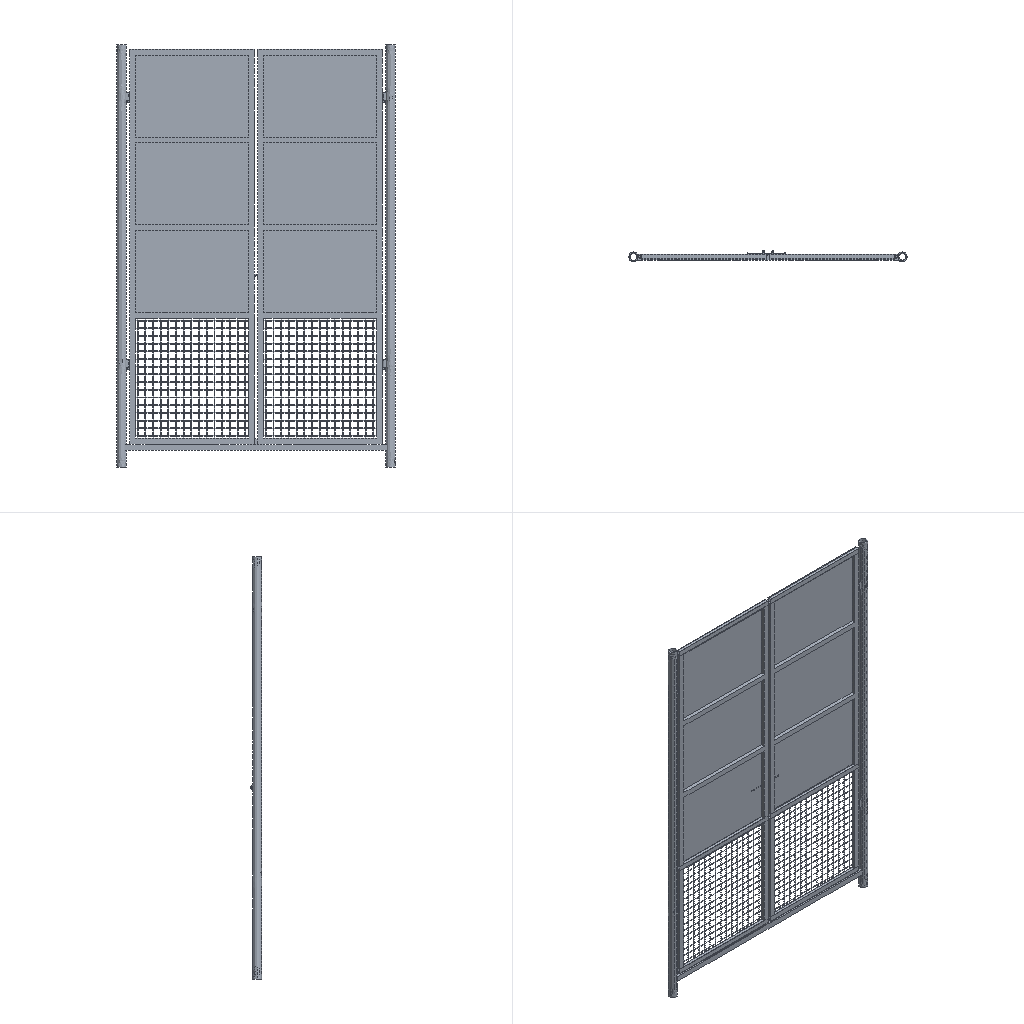Simulation study | ansys workbench
Ansys APDL input file, long lists of numbers shortened:
/batch
/config,noeldb,1     ! force off writing results to database
*get,_wallstrt,active,,time,wall
! ANSYS input file written by Workbench version 2022 R1
! File used for geometry attach:
/title,11111111--____ (C5)
! ****** Begin Custom Load Command Snippet ******
/COM, ACT Extensions:
/COM,     LSDYNA, 2021.1
/COM,
! ****** End   Custom Load Command Snippet ******
*DIM,_wb_ProjectScratch_dir,string,248
_wb_ProjectScratch_dir(1) = ''
*DIM,_wb_SolverFiles_dir,string,248
_wb_SolverFiles_dir(1) = ''
*DIM,_wb_userfiles_dir,string,248
_wb_userfiles_dir(1) = ''
/com,--- Data in consistent NMM units. See Solving Units in the help system for more information.
/units,MPA
/nopr
/wb,file,start              !  signify a WB generated input file
/prep7
! Turn off shape checking because checks already performed inside WB mesher.
! See help system for more information.
SHPP,OFF,,NOWARN
/nolist
etcon,set             ! allow ANSYS to choose best KEYOP's for 180x elements, resets any applicable keyopt to MAPDL defaults
/com,*********** Nodes for the whole assembly ***********
nblock,3,,286107
(1i9,3e20.9e3)
    12949     1.933800000E+03     1.900000000E+01    -1.195000000E+03
! (260097 more lines like these left out)
-1
/com,*********** Nodes for all Remote Points ***********
nblock,3
(1i9,3e20.9e3)
   280991     1.842299988E+03     1.800000000E+01    -2.097050049E+03
   280992     1.842299988E+03     1.800000000E+01    -2.097050049E+03
-1
/wb,elem,start            !  set before creation of elements
/com,*********** Elements for Body 1 "SYS-FreeParts|NONE[13]" ***********
et,1,187
eblock,19,solid,,50369
(19i9)
        1        1        1        1        0        0        0        0       10        0    25503    67432    85573    67447    85112    92001    92116    91995    91999
! (100737 more lines like these left out)
-1
/com,*********** Elements for Body 2 "SYS-FreeParts|NONE[14]" ***********
et,2,187
eblock,19,solid,,202
(19i9)
        2        2        2        2        0        0        0        0       10        0     1705    12989    12990    13041    12992    13285    13290    13287    13286
! (403 more lines like these left out)
-1
/com,*********** Elements for Body 3 "SYS-FreeParts|NONE[15]" ***********
et,3,187
eblock,19,solid,,2656
(19i9)
        3        3        3        3        0        0        0        0       10        0     2627    19012    19567    19821    19480    20721    23597    20722    20720
! (5311 more lines like these left out)
-1
/com,*********** Elements for Body 4 "SYS-FreeParts|NONE[16]" ***********
et,4,187
eblock,19,solid,,9942
(19i9)
        4        4        4        4        0        0        0        0       10        0     5611    26899    26916    28911    28178    31186    31316    31191    31190
! (19883 more lines like these left out)
-1
/com,*********** Elements for Body 5 "SYS-FreeParts|NONE[17]" ***********
et,5,187
eblock,19,solid,,9950
(19i9)
        5        5        5        5        0        0        0        0       10        0    15553    47411    47442    49475    47446    55304    55442    55306    55305
! (19899 more lines like these left out)
-1
/com,*********** Elements for Body 6 "SYS-FreeParts|NONE[18]" ***********
et,6,187
eblock,19,solid,,50302
(19i9)
        6        6        6        6        0        0        0        0       10        0    75872   179586   182598   192743   179592   229829   237337   229832   229827
! (100603 more lines like these left out)
-1
/wb,elem,end               !  done creating elements
/com,*********** Send User Defined Coordinate System(s) ***********
local,12,0,1842.3,18.,-2097.05,90.,0.,90.
csys,0
toffst,273.15,  ! Temperature offset from absolute zero
/com,*********** Set Reference Temperature ***********
tref,22.
/wb,mat,start              !  starting to send materials
/com,*********** Send Materials ***********
Temperature = 'TEMP' ! Temperature
MP,DENS,1,7.85e-09,	! tonne mm^-3
MP,ALPX,1,1.2e-05,	! C^-1
MP,C,1,434000000,	! mm^2 s^-2 C^-1
MP,KXX,1,60.5,	! tonne mm s^-3 C^-1
MP,RSVX,1,0.00017,	! ohm mm
MP,EX,1,200000,	! tonne s^-2 mm^-1
MP,NUXY,1,0.3,
MP,MURX,1,10000,
Temperature = 'TEMP' ! Temperature
MP,DENS,2,7.85e-09,	! tonne mm^-3
MP,ALPX,2,1.2e-05,	! C^-1
MP,C,2,434000000,	! mm^2 s^-2 C^-1
MP,KXX,2,60.5,	! tonne mm s^-3 C^-1
MP,RSVX,2,0.00017,	! ohm mm
MP,EX,2,200000,	! tonne s^-2 mm^-1
MP,NUXY,2,0.3,
MP,MURX,2,10000,
Temperature = 'TEMP' ! Temperature
MP,DENS,3,7.85e-09,	! tonne mm^-3
MP,ALPX,3,1.2e-05,	! C^-1
MP,C,3,434000000,	! mm^2 s^-2 C^-1
MP,KXX,3,60.5,	! tonne mm s^-3 C^-1
MP,RSVX,3,0.00017,	! ohm mm
MP,EX,3,200000,	! tonne s^-2 mm^-1
MP,NUXY,3,0.3,
MP,MURX,3,10000,
Temperature = 'TEMP' ! Temperature
MP,DENS,4,7.85e-09,	! tonne mm^-3
MP,ALPX,4,1.2e-05,	! C^-1
MP,C,4,434000000,	! mm^2 s^-2 C^-1
MP,KXX,4,60.5,	! tonne mm s^-3 C^-1
MP,RSVX,4,0.00017,	! ohm mm
MP,EX,4,200000,	! tonne s^-2 mm^-1
MP,NUXY,4,0.3,
MP,MURX,4,10000,
Temperature = 'TEMP' ! Temperature
MP,DENS,5,7.85e-09,	! tonne mm^-3
MP,ALPX,5,1.2e-05,	! C^-1
MP,C,5,434000000,	! mm^2 s^-2 C^-1
MP,KXX,5,60.5,	! tonne mm s^-3 C^-1
MP,RSVX,5,0.00017,	! ohm mm
MP,EX,5,200000,	! tonne s^-2 mm^-1
MP,NUXY,5,0.3,
MP,MURX,5,10000,
Temperature = 'TEMP' ! Temperature
MP,DENS,6,7.85e-09,	! tonne mm^-3
MP,ALPX,6,1.2e-05,	! C^-1
MP,C,6,434000000,	! mm^2 s^-2 C^-1
MP,KXX,6,60.5,	! tonne mm s^-3 C^-1
MP,RSVX,6,0.00017,	! ohm mm
MP,EX,6,200000,	! tonne s^-2 mm^-1
MP,NUXY,6,0.3,
MP,MURX,6,10000,
/wb,mat,end                !  done sending materials
!************************* Model Summary ********************
!SYS-FreeParts|NONE[13],	结构钢,	matid,	1
!SYS-FreeParts|NONE[14],	结构钢,	matid,	2
!SYS-FreeParts|NONE[15],	结构钢,	matid,	3
!SYS-FreeParts|NONE[16],	结构钢,	matid,	4
!SYS-FreeParts|NONE[17],	结构钢,	matid,	5
!SYS-FreeParts|NONE[18],	结构钢,	matid,	6
!************************* End Model Summary ********************
! get the diagonal of the bounding box. Needed later for other things
*get,_xmin,node,,mnloc,x
*get,_ymin,node,,mnloc,y
*get,_zmin,node,,mnloc,z
*get,_xmax,node,,mxloc,x
*get,_ymax,node,,mxloc,y
*get,_zmax,node,,mxloc,z
_ASMDIAG=(_xmax-_xmin)*(_xmax-_xmin)+(_ymax-_ymin)*(_ymax-_ymin)+(_zmax-_zmin)*(_zmax-_zmin)
_ASMDIAG=SQRT(_ASMDIAG)
/wb,contact,start          !  starting to send contact
/com,*********** Create Contact "摩擦的 - SYS-FreeParts|NONE[16] 至 SYS-FreeParts|NONE[18]" ***********
/com,            Real Constant Set For Above Contact Is 8 & 7
*set,tid,8
*set,cid,7
r,tid
r,cid
et,tid,170
et,cid,174
eblock,10,,,72
(15i9)
   222175        8        8        8        0    27051    27053    30075    30075    32307    32320    30075    32314
! (71 more lines like these left out)
-1
eblock,10,,,72
(15i9)
   222247        7        7        7        0    27051    27053    30075    30075    32307    32320    30075    32314
! (71 more lines like these left out)
-1
eblock,10,,,100
(15i9)
   222319        7        8        7        0   187204   177723   187206   187206   216670   216671   187206   266056
! (99 more lines like these left out)
-1
eblock,10,,,100
(15i9)
   222419        8        7        8        0   187204   177723   187206   187206   216670   216671   187206   266056
! (99 more lines like these left out)
-1
keyo,cid,8,2               ! auto create asymmetric contact (from Program Controlled setting)
keyo,cid,10,0              ! adjust contact stiffness each NR iteration (from Program Controlled setting)
keyo,cid,12,0              ! standard contact
mp,mu,cid,0.2       ! unitless
keyo,cid,18,1              ! small sliding turned on by application
keyo,cid,2,0               ! augmented Lagrange (from Program Controlled setting)
keyo,cid,4,0               ! on Gauss point (from Program Controlled setting)
keyo,cid,9,0               ! use real geometry with stepped effects
keyo,cid,7,0               ! No Prediction
rmod,tid,3,1.       ! FKN
rmod,tid,5,0.       ! ICONT
rmod,tid,6,0.       ! PINB
rmod,tid,10,0.      ! CNOF
rmod,tid,12,0.      ! FKT
rmod,tid,36,317     ! WB DSID
rmod,cid,3,1.       ! FKN
rmod,cid,5,0.       ! ICONT
rmod,cid,6,0.       ! PINB
rmod,cid,10,0.      ! CNOF
rmod,cid,12,0.      ! FKT
rmod,cid,36,317     ! WB DSID
/com,*********** Create Contact "摩擦的 - SYS-FreeParts|NONE[17] 至 SYS-FreeParts|NONE[13]" ***********
/com,            Real Constant Set For Above Contact Is 10 & 9
*set,tid,10
*set,cid,9
r,tid
r,cid
et,tid,170
et,cid,174
eblock,10,,,70
(15i9)
   222519       10       10       10        0    47052    47377    47057    47057    52390    52411    47057    52388
! (69 more lines like these left out)
-1
eblock,10,,,70
(15i9)
   222589        9        9        9        0    47052    47377    47057    47057    52390    52411    47057    52388
! (69 more lines like these left out)
-1
eblock,10,,,100
(15i9)
   222659        9       10        9        0    66805    66806    80026    80026    86117    86122    80026    86119
! (99 more lines like these left out)
-1
eblock,10,,,100
(15i9)
   222759       10        9       10        0    66805    66806    80026    80026    86117    86122    80026    86119
! (99 more lines like these left out)
-1
keyo,cid,8,2               ! auto create asymmetric contact (from Program Controlled setting)
keyo,cid,10,0              ! adjust contact stiffness each NR iteration (from Program Controlled setting)
keyo,cid,12,0              ! standard contact
keyo,cid,18,1              ! small sliding turned on by application
keyo,cid,2,0               ! augmented Lagrange (from Program Controlled setting)
keyo,cid,4,0               ! on Gauss point (from Program Controlled setting)
keyo,cid,9,0               ! use real geometry with stepped effects
keyo,cid,7,0               ! No Prediction
rmod,tid,3,1.       ! FKN
rmod,tid,5,0.       ! ICONT
rmod,tid,6,0.       ! PINB
rmod,tid,10,0.      ! CNOF
rmod,tid,12,0.      ! FKT
rmod,tid,36,320     ! WB DSID
rmod,cid,3,1.       ! FKN
rmod,cid,5,0.       ! ICONT
rmod,cid,6,0.       ! PINB
rmod,cid,10,0.      ! CNOF
rmod,cid,12,0.      ! FKT
rmod,cid,36,320     ! WB DSID
/com,*********** Create Contact "摩擦的 - SYS-FreeParts|NONE[14] 至 多个" ***********
/com,            Real Constant Set For Above Contact Is 12 & 11
*set,tid,12
*set,cid,11
r,tid
r,cid
et,tid,170
et,cid,174
eblock,10,,,168
(15i9)
   222859       12       12       12        0    12950    12985    12955    12955    13050    13067    12955    13049
! (167 more lines like these left out)
-1
eblock,10,,,168
(15i9)
   223027       11       11       11        0    12950    12985    12955    12955    13050    13067    12955    13049
! (167 more lines like these left out)
-1
eblock,10,,,64
(15i9)
   223195       11       12       11        0   178256   177288   178257   178257   212316   212317   178257   220315
! (63 more lines like these left out)
-1
eblock,10,,,64
(15i9)
   223259       12       11       12        0   178256   177288   178257   178257   212316   212317   178257   220315
! (63 more lines like these left out)
-1
keyo,cid,8,2               ! auto create asymmetric contact (from Program Controlled setting)
keyo,cid,10,0              ! adjust contact stiffness each NR iteration (from Program Controlled setting)
keyo,cid,12,0              ! standard contact
mp,mu,cid,0.6       ! unitless
keyo,cid,18,1              ! small sliding turned on by application
keyo,cid,2,0               ! augmented Lagrange (from Program Controlled setting)
keyo,cid,4,0               ! on Gauss point (from Program Controlled setting)
keyo,cid,9,0               ! use real geometry with stepped effects
keyo,cid,7,0               ! No Prediction
rmod,tid,3,1.       ! FKN
rmod,tid,5,0.       ! ICONT
rmod,tid,6,0.       ! PINB
rmod,tid,10,0.      ! CNOF
rmod,tid,12,0.      ! FKT
rmod,tid,36,323     ! WB DSID
rmod,cid,3,1.       ! FKN
rmod,cid,5,0.       ! ICONT
rmod,cid,6,0.       ! PINB
rmod,cid,10,0.      ! CNOF
rmod,cid,12,0.      ! FKT
rmod,cid,36,323     ! WB DSID
/com,*********** Create Contact "摩擦的 - SYS-FreeParts|NONE[15] 至 多个" ***********
/com,            Real Constant Set For Above Contact Is 14 & 13
*set,tid,14
*set,cid,13
r,tid
r,cid
et,tid,170
et,cid,174
eblock,10,,,24
(15i9)
   223323       14       14       14        0    18870    18868    19059    19059    19822    19824    19059    19831
! (23 more lines like these left out)
-1
eblock,10,,,24
(15i9)
   223347       13       13       13        0    18870    18868    19059    19059    19822    19824    19059    19831
! (23 more lines like these left out)
-1
eblock,10,,,7050
(15i9)
   223371       13       14       13        0    26896    26897    28181    28181    31166    31175    28181    31170
! (7049 more lines like these left out)
-1
eblock,10,,,7050
(15i9)
   230421       14       13       14        0    26896    26897    28181    28181    31166    31175    28181    31170
! (7049 more lines like these left out)
-1
keyo,cid,8,2               ! auto create asymmetric contact (from Program Controlled setting)
keyo,cid,10,0              ! adjust contact stiffness each NR iteration (from Program Controlled setting)
keyo,cid,12,0              ! standard contact
keyo,cid,18,1              ! small sliding turned on by application
keyo,cid,2,0               ! augmented Lagrange (from Program Controlled setting)
keyo,cid,4,0               ! on Gauss point (from Program Controlled setting)
keyo,cid,9,0               ! use real geometry with stepped effects
keyo,cid,7,0               ! No Prediction
rmod,tid,3,1.       ! FKN
rmod,tid,5,0.       ! ICONT
rmod,tid,6,0.       ! PINB
rmod,tid,10,0.      ! CNOF
rmod,tid,12,0.      ! FKT
rmod,tid,36,327     ! WB DSID
rmod,cid,3,1.       ! FKN
rmod,cid,5,0.       ! ICONT
rmod,cid,6,0.       ! PINB
rmod,cid,10,0.      ! CNOF
rmod,cid,12,0.      ! FKT
rmod,cid,36,327     ! WB DSID
nsel,all
esel,all
/wb,contact,end            !  done creating contacts
/golist
/wb,load,start             !  starting to send loads
/com,*********** Fixed Supports ***********
CMBLOCK,_FIXEDSU,NODE,      264
(8i10)
     26740     26741     26742     26743     26744     26745     26746     26747
! (32 more lines like these left out)
cmsel,s,_FIXEDSU
d,all,all
nsel,all
/com,*********** Create Remote Point "内部远程点 2" ***********
! -------- Remote Point Used by "固定的 - 接地 至 SYS-FreeParts|NONE[15]" --------
*set,tid,16
*set,cid,15
et,cid,174
et,tid,170
keyo,tid,2,1               ! Don't fix the pilot node
keyo,tid,4,111111
keyo,cid,12,5              ! Bonded Contact
keyo,cid,4,2               ! Rigid CERIG style load
keyo,cid,2,2               ! MPC style contact
eblock,10,,,375
(15i9)
   237471       15       15       15        0    18958    19587    18959    18959    20404    20411    18959    20401
! (374 more lines like these left out)
-1
*set,_npilot,280992
_npilot333=_npilot
type,tid
mat ,cid
real,cid
tshape,pilo
en,237846,_npilot
tshape
csys,12
nrot,280992
csys,0
/com,*********** Create Joint "固定的 - 接地 至 SYS-FreeParts|NONE[15]" ***********
/com,            Real Constant Set For Above Joint Is 17
! Joint Element Type Declaration and Definition using MPC184
*set,_jid,17
et,_jid,184
keyo,_jid,1,13          ! Fixed Joint
sectype,_jid, joint, weld, _wbjoint
secjoint,,12,12
mat,_jid
real,_jid
type,_jid
secnum,_jid
en,222174,,280992        ! body to ground joint
/com,*********** Define Force Using Surface Effect Elements ***********
local,13,0,0.,0.,0.,0.,0.,0.
csys,0
et,18,154
eblock,10,,,44
(15i9)
   237847       18       18       18       13   192145   192148   192151   192151   280121   280128   192151   280122
! (43 more lines like these left out)
-1
esel,s,type,,18
keyop,18,2,1                ! Apply load in local coordinate system
keyop,18,7,1                ! Use original area so load is constant in large deformation
esel,all
/gst,on,on
fini
*get,_numnode,node,0,count
*get,_numelem,elem,0,count
*get, _MAXELEMNUM, elem, 0, NUM, MAX
*get, _MAXNODENUM, node, 0, NUM, MAX
*get, _MAXELEMTYPE, etyp, 0, NUM, MAX
*get, _MAXREALCONST, real, 0, NUM, MAX
/go
/wb,load,end               !  done creating loads
/com,--- Number of total nodes = %_numnode%
/com,--- Number of contact elements = 15715
/com,--- Number of spring elements = 0
/com,--- Number of bearing elements = 0
/com,--- Number of solid elements = 123421
/com,--- Number of condensed parts = 0
/com,--- Number of total elements = %_numelem%
*get,_wallbsol,active,,time,wall
/com,****************************************************************************
/com,*************************    SOLUTION       ********************************
/com,****************************************************************************
/solu
antype,0                   ! static analysis
_thickRatio=0.167   ! Ratio of thick parts in the model
eqsl,sparse,,,,,1
cntr,print,1               ! print out contact info and also make no initial contact an error
dmpoption,emat,no             ! Don't combine emat file for DANSYS
dmpoption,esav,no             ! Don't combine esav file for DANSYS
nldiag,cont,iter           ! print out contact info each equilibrium iteration
rescontrol,define,last,last,,dele	   ! Program Controlled
/com,****************************************************
/com,******************* SOLVE FOR LS 1 OF 1 ****************
esel,s,type,,18
nsle
sfe,all,1,pres,1,0.
sfe,all,2,pres,1,6.00011508220545e-002
sfe,all,3,pres,1,0.
nsel,all
esel,all
/nopr
/gopr
autots,on                  ! Workbench Program Controlled automatic time stepping
nsub,5,20,1                ! due to presence of high frictional contact
time,1.
outres,erase
outres,all,none
outres,nsol,all,
outres,rsol,all
outres,eangl,all
outres,etmp,all
outres,veng,all
outres,strs,all,
outres,epel,all,
outres,eppl,all,
outres,cont,all,
/nopr
esel,s,type,,17
cm,_elmisc,elem
esel,all
/gopr
outres,misc,all,_elmisc
! *********** WB SOLVE COMMAND ***********
! check interactive state
*get,ANSINTER_,active,,int
*if,ANSINTER_,ne,0,then
/eof
*endif
solve
/com *************** Write FE CONNECTORS *********
CEWRITE,file,ce,,INTE
/com,****************************************************
/com,*************** FINISHED SOLVE FOR LS 1 *************
*get,_wallasol,active,,time,wall
/nopr
*get,_numnode,node,0,count
*get,_numelem,elem,0,count
*get, _MAXELEMNUM, elem, 0, NUM, MAX
*get, _MAXNODENUM, node, 0, NUM, MAX,,,INTERNAL
*get, _MAXELEMTYPE, etyp, 0, NUM, MAX
*get, _MAXREALCONST, real, 0, NUM, MAX
/gopr
/post1
xmlo,ENCODING,ISO-8859-1
xmlo,parm
/xml,parm,xml
fini
/gopr
*get,_walldone,active,,time,wall
_preptime=(_wallbsol-_wallstrt)*3600
_solvtime=(_wallasol-_wallbsol)*3600
_posttime=(_walldone-_wallasol)*3600
_totaltim=(_walldone-_wallstrt)*3600
*get,_dlbratio,active,0,solu,dlbr
*get,_combtime,active,0,solu,comb
*get,_ssmode,active,0,solu,ssmm
*get,_ndofs,active,0,solu,ndof
*get,_sol_end_time,active,0,set,time
*if,_sol_end_time,eq,1.,then
/fclean				!clean distributed files
*endif
/com,--- Total number of nodes = %_numnode%
/com,--- Total number of elements = %_numelem%
/com,--- Element load balance ratio = %_dlbratio%
/com,--- Time to combine distributed files = %_combtime%
/com,--- Sparse memory mode = %_ssmode%
/com,--- Number of DOF = %_ndofs%
/wb,file,end               ! done with WB generated input